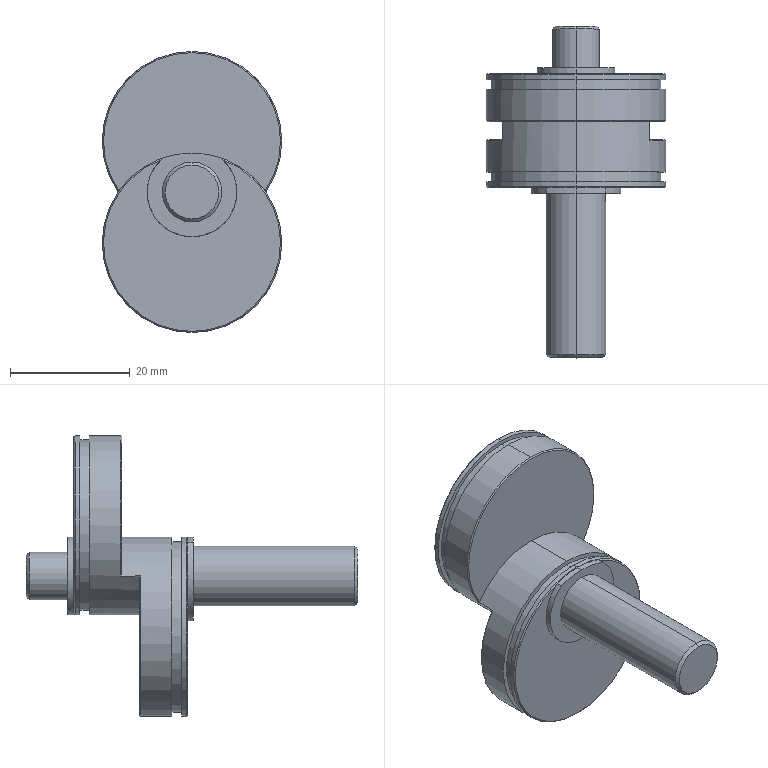Part | SolidWorks | features ICE 7, Chamfer 2, BaseBody 1 | 1 solid | 47 faces | box 30 x 55.5 x 47 mm | volume 14567 mm3 | cylinder 21 | cone 13 | plane 13 | commonest cylinder face diameters 30 x10 28.5 x4 8 x2 10 x2 13 x2 15 x1
STEP:
#1=CARTESIAN_POINT('',(0.,0.,-4.5));
#2=VERTEX_POINT('',#1);
#3=CARTESIAN_POINT('',(0.,0.,4.5));
#4=VERTEX_POINT('',#3);
#5=CARTESIAN_POINT('',(0.,0.,0.));
#6=DIRECTION('',(0.,-1.,0.));
#7=DIRECTION('',(0.,0.,-1.));
#8=AXIS2_PLACEMENT_3D('',#5,#6,#7);
#9=CIRCLE('',#8,4.5);
#10=EDGE_CURVE('',#2,#4,#9,.T.);
#11=ORIENTED_EDGE('',*,*,#10,.F.);
#12=CARTESIAN_POINT('',(0.,0.5,-5.));
#13=VERTEX_POINT('',#12);
#14=CARTESIAN_POINT('',(0.,0.,-4.5));
#15=DIRECTION('',(0.,0.7071,-0.7071));
#16=VECTOR('',#15,1000.);
#17=LINE('',#14,#16);
#18=EDGE_CURVE('',#2,#13,#17,.T.);
#19=ORIENTED_EDGE('',*,*,#18,.T.);
#20=CARTESIAN_POINT('',(0.,0.5,5.));
#21=VERTEX_POINT('',#20);
#22=CARTESIAN_POINT('',(0.,0.5,0.));
#23=DIRECTION('',(0.,1.,0.));
#24=DIRECTION('',(0.,0.,-1.));
#25=AXIS2_PLACEMENT_3D('',#22,#23,#24);
#26=CIRCLE('',#25,5.);
#27=EDGE_CURVE('',#21,#13,#26,.T.);
#28=ORIENTED_EDGE('',*,*,#27,.F.);
#29=CARTESIAN_POINT('',(0.,0.,4.5));
#30=DIRECTION('',(0.,0.7071,0.7071));
#31=VECTOR('',#30,1000.);
#32=LINE('',#29,#31);
#33=EDGE_CURVE('',#4,#21,#32,.T.);
#34=ORIENTED_EDGE('',*,*,#33,.F.);
#35=EDGE_LOOP('',(#11,#19,#28,#34));
#36=FACE_OUTER_BOUND('',#35,.T.);
#37=CARTESIAN_POINT('',(0.,0.,0.));
#38=DIRECTION('',(0.,1.,0.));
#39=DIRECTION('',(0.,0.,1.));
#40=AXIS2_PLACEMENT_3D('',#37,#38,#39);
#41=CONICAL_SURFACE('',#40,4.5,0.7854);
#42=ADVANCED_FACE('',(#36),#41,.T.);
#43=CARTESIAN_POINT('',(0.,55.5,3.5));
#44=VERTEX_POINT('',#43);
#45=CARTESIAN_POINT('',(0.,55.5,-3.5));
#46=VERTEX_POINT('',#45);
#47=CARTESIAN_POINT('',(0.,55.5,0.));
#48=DIRECTION('',(0.,1.,0.));
#49=DIRECTION('',(0.,0.,1.));
#50=AXIS2_PLACEMENT_3D('',#47,#48,#49);
#51=CIRCLE('',#50,3.5);
#52=EDGE_CURVE('',#44,#46,#51,.T.);
#53=ORIENTED_EDGE('',*,*,#52,.F.);
#54=CARTESIAN_POINT('',(0.,55.,4.));
#55=VERTEX_POINT('',#54);
#56=CARTESIAN_POINT('',(0.,55.5,3.5));
#57=DIRECTION('',(0.,-0.7071,0.7071));
#58=VECTOR('',#57,1000.);
#59=LINE('',#56,#58);
#60=EDGE_CURVE('',#44,#55,#59,.T.);
#61=ORIENTED_EDGE('',*,*,#60,.T.);
#62=CARTESIAN_POINT('',(0.,55.,-4.));
#63=VERTEX_POINT('',#62);
#64=CARTESIAN_POINT('',(0.,55.,0.));
#65=DIRECTION('',(0.,-1.,0.));
#66=DIRECTION('',(0.,0.,1.));
#67=AXIS2_PLACEMENT_3D('',#64,#65,#66);
#68=CIRCLE('',#67,4.);
#69=EDGE_CURVE('',#63,#55,#68,.T.);
#70=ORIENTED_EDGE('',*,*,#69,.F.);
#71=CARTESIAN_POINT('',(0.,55.5,-3.5));
#72=DIRECTION('',(0.,-0.7071,-0.7071));
#73=VECTOR('',#72,1000.);
#74=LINE('',#71,#73);
#75=EDGE_CURVE('',#46,#63,#74,.T.);
#76=ORIENTED_EDGE('',*,*,#75,.F.);
#77=EDGE_LOOP('',(#53,#61,#70,#76));
#78=FACE_OUTER_BOUND('',#77,.T.);
#79=CARTESIAN_POINT('',(0.,55.5,0.));
#80=DIRECTION('',(0.,-1.,0.));
#81=DIRECTION('',(0.,0.,-1.));
#82=AXIS2_PLACEMENT_3D('',#79,#80,#81);
#83=CONICAL_SURFACE('',#82,3.5,0.7854);
#84=ADVANCED_FACE('',(#78),#83,.T.);
#85=ORIENTED_EDGE('',*,*,#69,.T.);
#86=CARTESIAN_POINT('',(0.,48.5,4.));
#87=VERTEX_POINT('',#86);
#88=CARTESIAN_POINT('',(0.,55.5,4.));
#89=DIRECTION('',(0.,-1.,0.));
#90=VECTOR('',#89,1000.);
#91=LINE('',#88,#90);
#92=EDGE_CURVE('',#55,#87,#91,.T.);
#93=ORIENTED_EDGE('',*,*,#92,.T.);
#94=CARTESIAN_POINT('',(0.,48.5,-4.));
#95=VERTEX_POINT('',#94);
#96=CARTESIAN_POINT('',(0.,48.5,0.));
#97=DIRECTION('',(0.,1.,0.));
#98=DIRECTION('',(0.,0.,1.));
#99=AXIS2_PLACEMENT_3D('',#96,#97,#98);
#100=CIRCLE('',#99,4.);
#101=EDGE_CURVE('',#87,#95,#100,.T.);
#102=ORIENTED_EDGE('',*,*,#101,.T.);
#103=CARTESIAN_POINT('',(0.,55.5,-4.));
#104=DIRECTION('',(0.,-1.,0.));
#105=VECTOR('',#104,1000.);
#106=LINE('',#103,#105);
#107=EDGE_CURVE('',#63,#95,#106,.T.);
#108=ORIENTED_EDGE('',*,*,#107,.F.);
#109=EDGE_LOOP('',(#85,#93,#102,#108));
#110=FACE_OUTER_BOUND('',#109,.T.);
#111=CARTESIAN_POINT('',(0.,55.5,0.));
#112=DIRECTION('',(0.,-1.,0.));
#113=DIRECTION('',(0.,0.,-1.));
#114=AXIS2_PLACEMENT_3D('',#111,#112,#113);
#115=CYLINDRICAL_SURFACE('',#114,4.);
#116=ADVANCED_FACE('',(#110),#115,.T.);
#117=ORIENTED_EDGE('',*,*,#27,.T.);
#118=CARTESIAN_POINT('',(0.,27.5,-5.));
#119=VERTEX_POINT('',#118);
#120=CARTESIAN_POINT('',(0.,0.,-5.));
#121=DIRECTION('',(0.,1.,0.));
#122=VECTOR('',#121,1000.);
#123=LINE('',#120,#122);
#124=EDGE_CURVE('',#13,#119,#123,.T.);
#125=ORIENTED_EDGE('',*,*,#124,.T.);
#126=CARTESIAN_POINT('',(0.,27.5,5.));
#127=VERTEX_POINT('',#126);
#128=CARTESIAN_POINT('',(0.,27.5,0.));
#129=DIRECTION('',(0.,-1.,0.));
#130=DIRECTION('',(0.,0.,-1.));
#131=AXIS2_PLACEMENT_3D('',#128,#129,#130);
#132=CIRCLE('',#131,5.);
#133=EDGE_CURVE('',#119,#127,#132,.T.);
#134=ORIENTED_EDGE('',*,*,#133,.T.);
#135=CARTESIAN_POINT('',(0.,0.,5.));
#136=DIRECTION('',(0.,1.,0.));
#137=VECTOR('',#136,1000.);
#138=LINE('',#135,#137);
#139=EDGE_CURVE('',#21,#127,#138,.T.);
#140=ORIENTED_EDGE('',*,*,#139,.F.);
#141=EDGE_LOOP('',(#117,#125,#134,#140));
#142=FACE_OUTER_BOUND('',#141,.T.);
#143=CARTESIAN_POINT('',(0.,0.,0.));
#144=DIRECTION('',(0.,1.,0.));
#145=DIRECTION('',(0.,0.,1.));
#146=AXIS2_PLACEMENT_3D('',#143,#144,#145);
#147=CYLINDRICAL_SURFACE('',#146,5.);
#148=ADVANCED_FACE('',(#142),#147,.T.);
#149=CARTESIAN_POINT('',(0.,27.5,6.5));
#150=VERTEX_POINT('',#149);
#151=CARTESIAN_POINT('',(-4.902,27.5,5.676));
#152=VERTEX_POINT('',#151);
#153=CARTESIAN_POINT('',(0.,27.5,-8.5));
#154=DIRECTION('',(0.,-1.,0.));
#155=DIRECTION('',(0.,0.,1.));
#156=AXIS2_PLACEMENT_3D('',#153,#154,#155);
#157=CIRCLE('',#156,15.);
#158=EDGE_CURVE('',#150,#152,#157,.T.);
#159=ORIENTED_EDGE('',*,*,#158,.F.);
#160=CARTESIAN_POINT('',(0.,28.5,6.5));
#161=VERTEX_POINT('',#160);
#162=CARTESIAN_POINT('',(0.,27.5,6.5));
#163=DIRECTION('',(0.,1.,0.));
#164=VECTOR('',#163,1000.);
#165=LINE('',#162,#164);
#166=EDGE_CURVE('',#150,#161,#165,.T.);
#167=ORIENTED_EDGE('',*,*,#166,.T.);
#168=CARTESIAN_POINT('',(-4.902,28.5,5.676));
#169=VERTEX_POINT('',#168);
#170=CARTESIAN_POINT('',(0.,28.5,-8.5));
#171=DIRECTION('',(0.,-1.,0.));
#172=DIRECTION('',(0.,0.,1.));
#173=AXIS2_PLACEMENT_3D('',#170,#171,#172);
#174=CIRCLE('',#173,15.);
#175=EDGE_CURVE('',#161,#169,#174,.T.);
#176=ORIENTED_EDGE('',*,*,#175,.T.);
#177=CARTESIAN_POINT('',(-4.902,27.5,5.676));
#178=DIRECTION('',(0.,1.,0.));
#179=VECTOR('',#178,1000.);
#180=LINE('',#177,#179);
#181=EDGE_CURVE('',#152,#169,#180,.T.);
#182=ORIENTED_EDGE('',*,*,#181,.F.);
#183=EDGE_LOOP('',(#159,#167,#176,#182));
#184=FACE_OUTER_BOUND('',#183,.T.);
#185=CARTESIAN_POINT('',(0.,27.5,-8.5));
#186=DIRECTION('',(0.,1.,0.));
#187=DIRECTION('',(0.,0.,1.));
#188=AXIS2_PLACEMENT_3D('',#185,#186,#187);
#189=CYLINDRICAL_SURFACE('',#188,15.);
#190=ADVANCED_FACE('',(#184),#189,.T.);
#191=CARTESIAN_POINT('',(0.,28.5,-23.3));
#192=VERTEX_POINT('',#191);
#193=CARTESIAN_POINT('',(5.281,28.5,5.326));
#194=VERTEX_POINT('',#193);
#195=CARTESIAN_POINT('',(0.,28.5,-8.5));
#196=DIRECTION('',(0.,-1.,0.));
#197=DIRECTION('',(0.,0.,-1.));
#198=AXIS2_PLACEMENT_3D('',#195,#196,#197);
#199=CIRCLE('',#198,14.8);
#200=EDGE_CURVE('',#192,#194,#199,.T.);
#201=ORIENTED_EDGE('',*,*,#200,.F.);
#202=CARTESIAN_POINT('',(0.,28.7,-23.5));
#203=VERTEX_POINT('',#202);
#204=CARTESIAN_POINT('',(0.,28.7,-23.5));
#205=DIRECTION('',(0.,0.7071,-0.7071));
#206=VECTOR('',#205,1000.);
#207=LINE('',#204,#206);
#208=EDGE_CURVE('',#192,#203,#207,.T.);
#209=ORIENTED_EDGE('',*,*,#208,.T.);
#210=CARTESIAN_POINT('',(0.,28.7,6.5));
#211=VERTEX_POINT('',#210);
#212=CARTESIAN_POINT('',(0.,28.7,-8.5));
#213=DIRECTION('',(0.,1.,0.));
#214=DIRECTION('',(0.,0.,-1.));
#215=AXIS2_PLACEMENT_3D('',#212,#213,#214);
#216=CIRCLE('',#215,15.);
#217=EDGE_CURVE('',#211,#203,#216,.T.);
#218=ORIENTED_EDGE('',*,*,#217,.F.);
#219=CARTESIAN_POINT('',(0.,28.5,6.3));
#220=VERTEX_POINT('',#219);
#221=CARTESIAN_POINT('',(0.,28.7,6.5));
#222=DIRECTION('',(0.,0.7071,0.7071));
#223=VECTOR('',#222,1000.);
#224=LINE('',#221,#223);
#225=EDGE_CURVE('',#220,#211,#224,.T.);
#226=ORIENTED_EDGE('',*,*,#225,.F.);
#227=CARTESIAN_POINT('',(0.,28.5,-8.5));
#228=DIRECTION('',(0.,-1.,0.));
#229=DIRECTION('',(0.,0.,-1.));
#230=AXIS2_PLACEMENT_3D('',#227,#228,#229);
#231=CIRCLE('',#230,14.8);
#232=EDGE_CURVE('',#194,#220,#231,.T.);
#233=ORIENTED_EDGE('',*,*,#232,.F.);
#234=EDGE_LOOP('',(#201,#209,#218,#226,#233));
#235=FACE_OUTER_BOUND('',#234,.T.);
#236=CARTESIAN_POINT('',(0.,28.7,-8.5));
#237=DIRECTION('',(0.,1.,0.));
#238=DIRECTION('',(0.,0.,1.));
#239=AXIS2_PLACEMENT_3D('',#236,#237,#238);
#240=CONICAL_SURFACE('',#239,15.,0.7854);
#241=ADVANCED_FACE('',(#235),#240,.T.);
#242=ORIENTED_EDGE('',*,*,#217,.T.);
#243=CARTESIAN_POINT('',(0.,29.5,-23.5));
#244=VERTEX_POINT('',#243);
#245=CARTESIAN_POINT('',(0.,28.5,-23.5));
#246=DIRECTION('',(0.,1.,0.));
#247=VECTOR('',#246,1000.);
#248=LINE('',#245,#247);
#249=EDGE_CURVE('',#203,#244,#248,.T.);
#250=ORIENTED_EDGE('',*,*,#249,.T.);
#251=CARTESIAN_POINT('',(0.,29.5,6.5));
#252=VERTEX_POINT('',#251);
#253=CARTESIAN_POINT('',(0.,29.5,-8.5));
#254=DIRECTION('',(0.,1.,0.));
#255=DIRECTION('',(0.,0.,-1.));
#256=AXIS2_PLACEMENT_3D('',#253,#254,#255);
#257=CIRCLE('',#256,15.);
#258=EDGE_CURVE('',#252,#244,#257,.T.);
#259=ORIENTED_EDGE('',*,*,#258,.F.);
#260=CARTESIAN_POINT('',(0.,28.5,6.5));
#261=DIRECTION('',(0.,1.,0.));
#262=VECTOR('',#261,1000.);
#263=LINE('',#260,#262);
#264=EDGE_CURVE('',#211,#252,#263,.T.);
#265=ORIENTED_EDGE('',*,*,#264,.F.);
#266=EDGE_LOOP('',(#242,#250,#259,#265));
#267=FACE_OUTER_BOUND('',#266,.T.);
#268=CARTESIAN_POINT('',(0.,28.5,-8.5));
#269=DIRECTION('',(0.,1.,0.));
#270=DIRECTION('',(0.,0.,1.));
#271=AXIS2_PLACEMENT_3D('',#268,#269,#270);
#272=CYLINDRICAL_SURFACE('',#271,15.);
#273=ADVANCED_FACE('',(#267),#272,.T.);
#274=CARTESIAN_POINT('',(0.,29.5,-22.75));
#275=VERTEX_POINT('',#274);
#276=CARTESIAN_POINT('',(0.,29.5,5.75));
#277=VERTEX_POINT('',#276);
#278=CARTESIAN_POINT('',(0.,29.5,-8.5));
#279=DIRECTION('',(0.,-1.,0.));
#280=DIRECTION('',(0.,0.,-1.));
#281=AXIS2_PLACEMENT_3D('',#278,#279,#280);
#282=CIRCLE('',#281,14.25);
#283=EDGE_CURVE('',#275,#277,#282,.T.);
#284=ORIENTED_EDGE('',*,*,#283,.F.);
#285=CARTESIAN_POINT('',(0.,31.1,-22.75));
#286=VERTEX_POINT('',#285);
#287=CARTESIAN_POINT('',(0.,29.5,-22.75));
#288=DIRECTION('',(0.,1.,0.));
#289=VECTOR('',#288,1000.);
#290=LINE('',#287,#289);
#291=EDGE_CURVE('',#275,#286,#290,.T.);
#292=ORIENTED_EDGE('',*,*,#291,.T.);
#293=CARTESIAN_POINT('',(0.,31.1,5.75));
#294=VERTEX_POINT('',#293);
#295=CARTESIAN_POINT('',(0.,31.1,-8.5));
#296=DIRECTION('',(0.,-1.,0.));
#297=DIRECTION('',(0.,0.,-1.));
#298=AXIS2_PLACEMENT_3D('',#295,#296,#297);
#299=CIRCLE('',#298,14.25);
#300=EDGE_CURVE('',#286,#294,#299,.T.);
#301=ORIENTED_EDGE('',*,*,#300,.T.);
#302=CARTESIAN_POINT('',(0.,29.5,5.75));
#303=DIRECTION('',(0.,1.,0.));
#304=VECTOR('',#303,1000.);
#305=LINE('',#302,#304);
#306=EDGE_CURVE('',#277,#294,#305,.T.);
#307=ORIENTED_EDGE('',*,*,#306,.F.);
#308=EDGE_LOOP('',(#284,#292,#301,#307));
#309=FACE_OUTER_BOUND('',#308,.T.);
#310=CARTESIAN_POINT('',(0.,29.5,-8.5));
#311=DIRECTION('',(0.,1.,0.));
#312=DIRECTION('',(0.,0.,1.));
#313=AXIS2_PLACEMENT_3D('',#310,#311,#312);
#314=CYLINDRICAL_SURFACE('',#313,14.25);
#315=ADVANCED_FACE('',(#309),#314,.T.);
#316=CARTESIAN_POINT('',(14.8,47.5,8.5));
#317=VERTEX_POINT('',#316);
#318=CARTESIAN_POINT('',(-14.8,47.5,8.5));
#319=VERTEX_POINT('',#318);
#320=CARTESIAN_POINT('',(0.,47.5,8.5));
#321=DIRECTION('',(0.,-1.,0.));
#322=DIRECTION('',(1.,0.,0.));
#323=AXIS2_PLACEMENT_3D('',#320,#321,#322);
#324=CIRCLE('',#323,14.8);
#325=EDGE_CURVE('',#317,#319,#324,.T.);
#326=ORIENTED_EDGE('',*,*,#325,.T.);
#327=CARTESIAN_POINT('',(-15.,47.3,8.5));
#328=VERTEX_POINT('',#327);
#329=CARTESIAN_POINT('',(-15.,47.3,8.5));
#330=DIRECTION('',(-0.7071,-0.7071,0.));
#331=VECTOR('',#330,1000.);
#332=LINE('',#329,#331);
#333=EDGE_CURVE('',#319,#328,#332,.T.);
#334=ORIENTED_EDGE('',*,*,#333,.T.);
#335=CARTESIAN_POINT('',(0.,47.3,23.5));
#336=VERTEX_POINT('',#335);
#337=CARTESIAN_POINT('',(0.,47.3,8.5));
#338=DIRECTION('',(0.,1.,0.));
#339=DIRECTION('',(0.,0.,-1.));
#340=AXIS2_PLACEMENT_3D('',#337,#338,#339);
#341=CIRCLE('',#340,15.);
#342=EDGE_CURVE('',#328,#336,#341,.T.);
#343=ORIENTED_EDGE('',*,*,#342,.T.);
#344=CARTESIAN_POINT('',(15.,47.3,8.5));
#345=VERTEX_POINT('',#344);
#346=CARTESIAN_POINT('',(0.,47.3,8.5));
#347=DIRECTION('',(0.,1.,0.));
#348=DIRECTION('',(0.,0.,-1.));
#349=AXIS2_PLACEMENT_3D('',#346,#347,#348);
#350=CIRCLE('',#349,15.);
#351=EDGE_CURVE('',#336,#345,#350,.T.);
#352=ORIENTED_EDGE('',*,*,#351,.T.);
#353=CARTESIAN_POINT('',(15.,47.3,8.5));
#354=DIRECTION('',(0.7071,-0.7071,0.));
#355=VECTOR('',#354,1000.);
#356=LINE('',#353,#355);
#357=EDGE_CURVE('',#317,#345,#356,.T.);
#358=ORIENTED_EDGE('',*,*,#357,.F.);
#359=EDGE_LOOP('',(#326,#334,#343,#352,#358));
#360=FACE_OUTER_BOUND('',#359,.T.);
#361=CARTESIAN_POINT('',(0.,47.3,8.5));
#362=DIRECTION('',(0.,-1.,0.));
#363=DIRECTION('',(1.,0.,0.));
#364=AXIS2_PLACEMENT_3D('',#361,#362,#363);
#365=CONICAL_SURFACE('',#364,15.,0.7854);
#366=ADVANCED_FACE('',(#360),#365,.T.);
#367=CARTESIAN_POINT('',(2.106,47.5,-6.149));
#368=VERTEX_POINT('',#367);
#369=CARTESIAN_POINT('',(0.,47.5,8.5));
#370=DIRECTION('',(0.,-1.,0.));
#371=DIRECTION('',(1.,0.,0.));
#372=AXIS2_PLACEMENT_3D('',#369,#370,#371);
#373=CIRCLE('',#372,14.8);
#374=EDGE_CURVE('',#368,#317,#373,.T.);
#375=ORIENTED_EDGE('',*,*,#374,.T.);
#376=ORIENTED_EDGE('',*,*,#357,.T.);
#377=CARTESIAN_POINT('',(0.0001635,47.3,-6.5));
#378=VERTEX_POINT('',#377);
#379=CARTESIAN_POINT('',(0.,47.3,8.5));
#380=DIRECTION('',(0.,1.,0.));
#381=DIRECTION('',(0.,0.,-1.));
#382=AXIS2_PLACEMENT_3D('',#379,#380,#381);
#383=CIRCLE('',#382,15.);
#384=EDGE_CURVE('',#345,#378,#383,.T.);
#385=ORIENTED_EDGE('',*,*,#384,.T.);
#386=CARTESIAN_POINT('',(0.0001635,47.3,-6.5));
#387=CARTESIAN_POINT('',(0.7279,47.3,-6.5));
#388=CARTESIAN_POINT('',(1.429,47.367,-6.381));
#389=CARTESIAN_POINT('',(2.106,47.5,-6.149));
#390=B_SPLINE_CURVE_WITH_KNOTS('',3,(#386,#387,#388,#389),.UNSPECIFIED.,.F.,.F.,(4,4),(0.,0.002144),.UNSPECIFIED.);
#391=EDGE_CURVE('',#378,#368,#390,.T.);
#392=ORIENTED_EDGE('',*,*,#391,.T.);
#393=EDGE_LOOP('',(#375,#376,#385,#392));
#394=FACE_OUTER_BOUND('',#393,.T.);
#395=CARTESIAN_POINT('',(0.,47.3,8.5));
#396=DIRECTION('',(0.,-1.,0.));
#397=DIRECTION('',(1.,0.,0.));
#398=AXIS2_PLACEMENT_3D('',#395,#396,#397);
#399=CONICAL_SURFACE('',#398,15.,0.7854);
#400=ADVANCED_FACE('',(#394),#399,.T.);
#401=ORIENTED_EDGE('',*,*,#351,.F.);
#402=CARTESIAN_POINT('',(0.,46.5,23.5));
#403=VERTEX_POINT('',#402);
#404=CARTESIAN_POINT('',(0.,47.5,23.5));
#405=DIRECTION('',(0.,-1.,0.));
#406=VECTOR('',#405,1000.);
#407=LINE('',#404,#406);
#408=EDGE_CURVE('',#336,#403,#407,.T.);
#409=ORIENTED_EDGE('',*,*,#408,.T.);
#410=CARTESIAN_POINT('',(0.,46.5,-6.5));
#411=VERTEX_POINT('',#410);
#412=CARTESIAN_POINT('',(0.,46.5,8.5));
#413=DIRECTION('',(0.,1.,0.));
#414=DIRECTION('',(0.,0.,-1.));
#415=AXIS2_PLACEMENT_3D('',#412,#413,#414);
#416=CIRCLE('',#415,15.);
#417=EDGE_CURVE('',#403,#411,#416,.T.);
#418=ORIENTED_EDGE('',*,*,#417,.T.);
#419=CARTESIAN_POINT('',(0.,47.3,-6.5));
#420=VERTEX_POINT('',#419);
#421=CARTESIAN_POINT('',(0.,47.5,-6.5));
#422=DIRECTION('',(0.,-1.,0.));
#423=VECTOR('',#422,1000.);
#424=LINE('',#421,#423);
#425=EDGE_CURVE('',#420,#411,#424,.T.);
#426=ORIENTED_EDGE('',*,*,#425,.F.);
#427=CARTESIAN_POINT('',(0.,47.3,8.5));
#428=DIRECTION('',(0.,1.,0.));
#429=DIRECTION('',(-0.000000001,0.,-1.));
#430=AXIS2_PLACEMENT_3D('',#427,#428,#429);
#431=CIRCLE('',#430,15.);
#432=EDGE_CURVE('',#378,#420,#431,.T.);
#433=ORIENTED_EDGE('',*,*,#432,.F.);
#434=ORIENTED_EDGE('',*,*,#384,.F.);
#435=EDGE_LOOP('',(#401,#409,#418,#426,#433,#434));
#436=FACE_OUTER_BOUND('',#435,.T.);
#437=CARTESIAN_POINT('',(0.,47.5,8.5));
#438=DIRECTION('',(0.,-1.,0.));
#439=DIRECTION('',(0.,0.,-1.));
#440=AXIS2_PLACEMENT_3D('',#437,#438,#439);
#441=CYLINDRICAL_SURFACE('',#440,15.);
#442=ADVANCED_FACE('',(#436),#441,.T.);
#443=CARTESIAN_POINT('',(0.,44.9,22.75));
#444=VERTEX_POINT('',#443);
#445=CARTESIAN_POINT('',(0.,44.9,-5.75));
#446=VERTEX_POINT('',#445);
#447=CARTESIAN_POINT('',(0.,44.9,8.5));
#448=DIRECTION('',(0.,1.,0.));
#449=DIRECTION('',(0.,0.,1.));
#450=AXIS2_PLACEMENT_3D('',#447,#448,#449);
#451=CIRCLE('',#450,14.25);
#452=EDGE_CURVE('',#444,#446,#451,.T.);
#453=ORIENTED_EDGE('',*,*,#452,.T.);
#454=CARTESIAN_POINT('',(0.,46.5,-5.75));
#455=VERTEX_POINT('',#454);
#456=CARTESIAN_POINT('',(0.,46.5,-5.75));
#457=DIRECTION('',(0.,1.,0.));
#458=VECTOR('',#457,1000.);
#459=LINE('',#456,#458);
#460=EDGE_CURVE('',#446,#455,#459,.T.);
#461=ORIENTED_EDGE('',*,*,#460,.T.);
#462=CARTESIAN_POINT('',(0.,46.5,22.75));
#463=VERTEX_POINT('',#462);
#464=CARTESIAN_POINT('',(0.,46.5,8.5));
#465=DIRECTION('',(0.,-1.,0.));
#466=DIRECTION('',(0.,0.,1.));
#467=AXIS2_PLACEMENT_3D('',#464,#465,#466);
#468=CIRCLE('',#467,14.25);
#469=EDGE_CURVE('',#455,#463,#468,.T.);
#470=ORIENTED_EDGE('',*,*,#469,.T.);
#471=CARTESIAN_POINT('',(0.,46.5,22.75));
#472=DIRECTION('',(0.,1.,0.));
#473=VECTOR('',#472,1000.);
#474=LINE('',#471,#473);
#475=EDGE_CURVE('',#444,#463,#474,.T.);
#476=ORIENTED_EDGE('',*,*,#475,.F.);
#477=EDGE_LOOP('',(#453,#461,#470,#476));
#478=FACE_OUTER_BOUND('',#477,.T.);
#479=CARTESIAN_POINT('',(0.,46.5,8.5));
#480=DIRECTION('',(0.,1.,0.));
#481=DIRECTION('',(0.,0.,1.));
#482=AXIS2_PLACEMENT_3D('',#479,#480,#481);
#483=CYLINDRICAL_SURFACE('',#482,14.25);
#484=ADVANCED_FACE('',(#478),#483,.T.);
#485=CARTESIAN_POINT('',(0.,44.9,23.5));
#486=VERTEX_POINT('',#485);
#487=CARTESIAN_POINT('',(0.,44.9,-6.5));
#488=VERTEX_POINT('',#487);
#489=CARTESIAN_POINT('',(0.,44.9,8.5));
#490=DIRECTION('',(0.,1.,0.));
#491=DIRECTION('',(0.,0.,-1.));
#492=AXIS2_PLACEMENT_3D('',#489,#490,#491);
#493=CIRCLE('',#492,15.);
#494=EDGE_CURVE('',#486,#488,#493,.T.);
#495=ORIENTED_EDGE('',*,*,#494,.F.);
#496=CARTESIAN_POINT('',(0.,39.7,23.5));
#497=VERTEX_POINT('',#496);
#498=CARTESIAN_POINT('',(0.,47.5,23.5));
#499=DIRECTION('',(0.,-1.,0.));
#500=VECTOR('',#499,1000.);
#501=LINE('',#498,#500);
#502=EDGE_CURVE('',#486,#497,#501,.T.);
#503=ORIENTED_EDGE('',*,*,#502,.T.);
#504=CARTESIAN_POINT('',(12.359,39.7,0.));
#505=VERTEX_POINT('',#504);
#506=CARTESIAN_POINT('',(0.,39.7,8.5));
#507=DIRECTION('',(0.,1.,0.));
#508=DIRECTION('',(0.,0.,-1.));
#509=AXIS2_PLACEMENT_3D('',#506,#507,#508);
#510=CIRCLE('',#509,15.);
#511=EDGE_CURVE('',#497,#505,#510,.T.);
#512=ORIENTED_EDGE('',*,*,#511,.T.);
#513=CARTESIAN_POINT('',(12.359,36.3,0.));
#514=VERTEX_POINT('',#513);
#515=CARTESIAN_POINT('',(12.359,47.5,0.));
#516=DIRECTION('',(0.,-1.,0.));
#517=VECTOR('',#516,1000.);
#518=LINE('',#515,#517);
#519=EDGE_CURVE('',#505,#514,#518,.T.);
#520=ORIENTED_EDGE('',*,*,#519,.T.);
#521=CARTESIAN_POINT('',(12.237,36.5,-0.1753));
#522=VERTEX_POINT('',#521);
#523=CARTESIAN_POINT('',(12.237,36.5,-0.1753));
#524=CARTESIAN_POINT('',(12.278,36.433,-0.1172));
#525=CARTESIAN_POINT('',(12.319,36.367,-0.05877));
#526=CARTESIAN_POINT('',(12.359,36.3,0.));
#527=B_SPLINE_CURVE_WITH_KNOTS('',3,(#523,#524,#525,#526),.UNSPECIFIED.,.F.,.F.,(4,4),(0.,0.0002928),.UNSPECIFIED.);
#528=EDGE_CURVE('',#522,#514,#527,.T.);
#529=ORIENTED_EDGE('',*,*,#528,.F.);
#530=CARTESIAN_POINT('',(0.,36.5,-6.5));
#531=VERTEX_POINT('',#530);
#532=CARTESIAN_POINT('',(0.,36.5,8.5));
#533=DIRECTION('',(0.,1.,0.));
#534=DIRECTION('',(0.,0.,-1.));
#535=AXIS2_PLACEMENT_3D('',#532,#533,#534);
#536=CIRCLE('',#535,15.);
#537=EDGE_CURVE('',#522,#531,#536,.T.);
#538=ORIENTED_EDGE('',*,*,#537,.T.);
#539=CARTESIAN_POINT('',(0.,47.5,-6.5));
#540=DIRECTION('',(0.,-1.,0.));
#541=VECTOR('',#540,1000.);
#542=LINE('',#539,#541);
#543=EDGE_CURVE('',#488,#531,#542,.T.);
#544=ORIENTED_EDGE('',*,*,#543,.F.);
#545=EDGE_LOOP('',(#495,#503,#512,#520,#529,#538,#544));
#546=FACE_OUTER_BOUND('',#545,.T.);
#547=CARTESIAN_POINT('',(0.,47.5,8.5));
#548=DIRECTION('',(0.,-1.,0.));
#549=DIRECTION('',(0.,0.,-1.));
#550=AXIS2_PLACEMENT_3D('',#547,#548,#549);
#551=CYLINDRICAL_SURFACE('',#550,15.);
#552=ADVANCED_FACE('',(#546),#551,.T.);
#553=CARTESIAN_POINT('',(-12.237,39.5,0.1753));
#554=VERTEX_POINT('',#553);
#555=CARTESIAN_POINT('',(0.,39.5,23.3));
#556=VERTEX_POINT('',#555);
#557=CARTESIAN_POINT('',(0.,39.5,8.5));
#558=DIRECTION('',(0.,1.,0.));
#559=DIRECTION('',(0.,0.,1.));
#560=AXIS2_PLACEMENT_3D('',#557,#558,#559);
#561=CIRCLE('',#560,14.8);
#562=EDGE_CURVE('',#554,#556,#561,.T.);
#563=ORIENTED_EDGE('',*,*,#562,.T.);
#564=CARTESIAN_POINT('',(0.,39.7,23.5));
#565=DIRECTION('',(0.,0.7071,0.7071));
#566=VECTOR('',#565,1000.);
#567=LINE('',#564,#566);
#568=EDGE_CURVE('',#556,#497,#567,.T.);
#569=ORIENTED_EDGE('',*,*,#568,.T.);
#570=CARTESIAN_POINT('',(-12.359,39.7,0.));
#571=VERTEX_POINT('',#570);
#572=CARTESIAN_POINT('',(0.,39.7,8.5));
#573=DIRECTION('',(0.,1.,0.));
#574=DIRECTION('',(0.,0.,-1.));
#575=AXIS2_PLACEMENT_3D('',#572,#573,#574);
#576=CIRCLE('',#575,15.);
#577=EDGE_CURVE('',#571,#497,#576,.T.);
#578=ORIENTED_EDGE('',*,*,#577,.F.);
#579=CARTESIAN_POINT('',(-12.359,39.7,0.));
#580=CARTESIAN_POINT('',(-12.319,39.633,0.05877));
#581=CARTESIAN_POINT('',(-12.278,39.567,0.1172));
#582=CARTESIAN_POINT('',(-12.237,39.5,0.1753));
#583=B_SPLINE_CURVE_WITH_KNOTS('',3,(#579,#580,#581,#582),.UNSPECIFIED.,.F.,.F.,(4,4),(0.,0.0002928),.UNSPECIFIED.);
#584=EDGE_CURVE('',#571,#554,#583,.T.);
#585=ORIENTED_EDGE('',*,*,#584,.T.);
#586=EDGE_LOOP('',(#563,#569,#578,#585));
#587=FACE_OUTER_BOUND('',#586,.T.);
#588=CARTESIAN_POINT('',(0.,39.7,8.5));
#589=DIRECTION('',(0.,1.,0.));
#590=DIRECTION('',(0.,0.,1.));
#591=AXIS2_PLACEMENT_3D('',#588,#589,#590);
#592=CONICAL_SURFACE('',#591,15.,0.7854);
#593=ADVANCED_FACE('',(#587),#592,.T.);
#594=CARTESIAN_POINT('',(-12.237,36.5,-0.1753));
#595=VERTEX_POINT('',#594);
#596=CARTESIAN_POINT('',(0.,36.5,-23.3));
#597=VERTEX_POINT('',#596);
#598=CARTESIAN_POINT('',(0.,36.5,-8.5));
#599=DIRECTION('',(0.,-1.,0.));
#600=DIRECTION('',(0.,0.,-1.));
#601=AXIS2_PLACEMENT_3D('',#598,#599,#600);
#602=CIRCLE('',#601,14.8);
#603=EDGE_CURVE('',#595,#597,#602,.T.);
#604=ORIENTED_EDGE('',*,*,#603,.T.);
#605=CARTESIAN_POINT('',(0.,36.3,-23.5));
#606=VERTEX_POINT('',#605);
#607=CARTESIAN_POINT('',(0.,36.3,-23.5));
#608=DIRECTION('',(0.,-0.7071,-0.7071));
#609=VECTOR('',#608,1000.);
#610=LINE('',#607,#609);
#611=EDGE_CURVE('',#597,#606,#610,.T.);
#612=ORIENTED_EDGE('',*,*,#611,.T.);
#613=CARTESIAN_POINT('',(-12.359,36.3,0.));
#614=VERTEX_POINT('',#613);
#615=CARTESIAN_POINT('',(0.,36.3,-8.5));
#616=DIRECTION('',(0.,1.,0.));
#617=DIRECTION('',(0.,0.,-1.));
#618=AXIS2_PLACEMENT_3D('',#615,#616,#617);
#619=CIRCLE('',#618,15.);
#620=EDGE_CURVE('',#606,#614,#619,.T.);
#621=ORIENTED_EDGE('',*,*,#620,.T.);
#622=CARTESIAN_POINT('',(-12.237,36.5,-0.1753));
#623=CARTESIAN_POINT('',(-12.278,36.433,-0.1172));
#624=CARTESIAN_POINT('',(-12.319,36.367,-0.05877));
#625=CARTESIAN_POINT('',(-12.359,36.3,0.));
#626=B_SPLINE_CURVE_WITH_KNOTS('',3,(#622,#623,#624,#625),.UNSPECIFIED.,.F.,.F.,(4,4),(0.,0.0002928),.UNSPECIFIED.);
#627=EDGE_CURVE('',#595,#614,#626,.T.);
#628=ORIENTED_EDGE('',*,*,#627,.F.);
#629=EDGE_LOOP('',(#604,#612,#621,#628));
#630=FACE_OUTER_BOUND('',#629,.T.);
#631=CARTESIAN_POINT('',(0.,36.3,-8.5));
#632=DIRECTION('',(0.,-1.,0.));
#633=DIRECTION('',(0.,0.,-1.));
#634=AXIS2_PLACEMENT_3D('',#631,#632,#633);
#635=CONICAL_SURFACE('',#634,15.,0.7854);
#636=ADVANCED_FACE('',(#630),#635,.T.);
#637=CARTESIAN_POINT('',(0.,47.3,-6.5));
#638=VERTEX_POINT('',#637);
#639=CARTESIAN_POINT('',(0.0001635,47.3,-6.5));
#640=CARTESIAN_POINT('',(0.000109,47.3,-6.5));
#641=CARTESIAN_POINT('',(0.0000545,47.3,-6.5));
#642=CARTESIAN_POINT('',(0.,47.3,-6.5));
#643=B_SPLINE_CURVE_WITH_KNOTS('',3,(#639,#640,#641,#642),.UNSPECIFIED.,.F.,.F.,(4,4),(0.,0.000000161),.UNSPECIFIED.);
#644=EDGE_CURVE('',#378,#638,#643,.T.);
#645=ORIENTED_EDGE('',*,*,#644,.T.);
#646=CARTESIAN_POINT('',(0.,48.5,-6.5));
#647=VERTEX_POINT('',#646);
#648=CARTESIAN_POINT('',(0.,48.5,-6.5));
#649=DIRECTION('',(0.,1.,0.));
#650=VECTOR('',#649,1000.);
#651=LINE('',#648,#650);
#652=EDGE_CURVE('',#638,#647,#651,.T.);
#653=ORIENTED_EDGE('',*,*,#652,.T.);
#654=CARTESIAN_POINT('',(0.,48.5,6.5));
#655=VERTEX_POINT('',#654);
#656=CARTESIAN_POINT('',(0.,48.5,0.));
#657=DIRECTION('',(0.,1.,0.));
#658=DIRECTION('',(0.,0.,1.));
#659=AXIS2_PLACEMENT_3D('',#656,#657,#658);
#660=CIRCLE('',#659,6.5);
#661=EDGE_CURVE('',#655,#647,#660,.T.);
#662=ORIENTED_EDGE('',*,*,#661,.F.);
#663=CARTESIAN_POINT('',(0.,47.5,6.5));
#664=VERTEX_POINT('',#663);
#665=CARTESIAN_POINT('',(0.,48.5,6.5));
#666=DIRECTION('',(0.,1.,0.));
#667=VECTOR('',#666,1000.);
#668=LINE('',#665,#667);
#669=EDGE_CURVE('',#664,#655,#668,.T.);
#670=ORIENTED_EDGE('',*,*,#669,.F.);
#671=CARTESIAN_POINT('',(0.,47.5,0.));
#672=DIRECTION('',(0.,1.,0.));
#673=DIRECTION('',(0.,0.,-1.));
#674=AXIS2_PLACEMENT_3D('',#671,#672,#673);
#675=CIRCLE('',#674,6.5);
#676=EDGE_CURVE('',#664,#368,#675,.T.);
#677=ORIENTED_EDGE('',*,*,#676,.T.);
#678=ORIENTED_EDGE('',*,*,#391,.F.);
#679=EDGE_LOOP('',(#645,#653,#662,#670,#677,#678));
#680=FACE_OUTER_BOUND('',#679,.T.);
#681=CARTESIAN_POINT('',(0.,48.5,0.));
#682=DIRECTION('',(0.,1.,0.));
#683=DIRECTION('',(0.,0.,1.));
#684=AXIS2_PLACEMENT_3D('',#681,#682,#683);
#685=CYLINDRICAL_SURFACE('',#684,6.5);
#686=ADVANCED_FACE('',(#680),#685,.T.);
#687=CARTESIAN_POINT('',(12.237,39.5,0.1753));
#688=VERTEX_POINT('',#687);
#689=CARTESIAN_POINT('',(0.,39.5,6.5));
#690=VERTEX_POINT('',#689);
#691=CARTESIAN_POINT('',(0.,39.5,-8.5));
#692=DIRECTION('',(0.,-1.,0.));
#693=DIRECTION('',(0.,0.,-1.));
#694=AXIS2_PLACEMENT_3D('',#691,#692,#693);
#695=CIRCLE('',#694,15.);
#696=EDGE_CURVE('',#688,#690,#695,.T.);
#697=ORIENTED_EDGE('',*,*,#696,.T.);
#698=CARTESIAN_POINT('',(0.,31.1,6.5));
#699=VERTEX_POINT('',#698);
#700=CARTESIAN_POINT('',(0.,39.5,6.5));
#701=DIRECTION('',(0.,-1.,0.));
#702=VECTOR('',#701,1000.);
#703=LINE('',#700,#702);
#704=EDGE_CURVE('',#690,#699,#703,.T.);
#705=ORIENTED_EDGE('',*,*,#704,.T.);
#706=CARTESIAN_POINT('',(0.,31.1,-23.5));
#707=VERTEX_POINT('',#706);
#708=CARTESIAN_POINT('',(0.,31.1,-8.5));
#709=DIRECTION('',(0.,-1.,0.));
#710=DIRECTION('',(0.,0.,-1.));
#711=AXIS2_PLACEMENT_3D('',#708,#709,#710);
#712=CIRCLE('',#711,15.);
#713=EDGE_CURVE('',#707,#699,#712,.T.);
#714=ORIENTED_EDGE('',*,*,#713,.F.);
#715=CARTESIAN_POINT('',(0.,39.5,-23.5));
#716=DIRECTION('',(0.,-1.,0.));
#717=VECTOR('',#716,1000.);
#718=LINE('',#715,#717);
#719=EDGE_CURVE('',#606,#707,#718,.T.);
#720=ORIENTED_EDGE('',*,*,#719,.F.);
#721=CARTESIAN_POINT('',(0.,36.3,-8.5));
#722=DIRECTION('',(0.,1.,0.));
#723=DIRECTION('',(0.,0.,-1.));
#724=AXIS2_PLACEMENT_3D('',#721,#722,#723);
#725=CIRCLE('',#724,15.);
#726=EDGE_CURVE('',#514,#606,#725,.T.);
#727=ORIENTED_EDGE('',*,*,#726,.F.);
#728=ORIENTED_EDGE('',*,*,#519,.F.);
#729=CARTESIAN_POINT('',(12.359,39.7,0.));
#730=CARTESIAN_POINT('',(12.319,39.633,0.05877));
#731=CARTESIAN_POINT('',(12.278,39.567,0.1172));
#732=CARTESIAN_POINT('',(12.237,39.5,0.1753));
#733=B_SPLINE_CURVE_WITH_KNOTS('',3,(#729,#730,#731,#732),.UNSPECIFIED.,.F.,.F.,(4,4),(0.,0.0002928),.UNSPECIFIED.);
#734=EDGE_CURVE('',#505,#688,#733,.T.);
#735=ORIENTED_EDGE('',*,*,#734,.T.);
#736=EDGE_LOOP('',(#697,#705,#714,#720,#727,#728,#735));
#737=FACE_OUTER_BOUND('',#736,.T.);
#738=CARTESIAN_POINT('',(0.,39.5,-8.5));
#739=DIRECTION('',(0.,-1.,0.));
#740=DIRECTION('',(0.,0.,-1.));
#741=AXIS2_PLACEMENT_3D('',#738,#739,#740);
#742=CYLINDRICAL_SURFACE('',#741,15.);
#743=ADVANCED_FACE('',(#737),#742,.T.);
#744=CARTESIAN_POINT('',(-2.106,47.5,-6.149));
#745=VERTEX_POINT('',#744);
#746=CARTESIAN_POINT('',(0.,47.5,0.));
#747=DIRECTION('',(0.,1.,0.));
#748=DIRECTION('',(0.,0.,-1.));
#749=AXIS2_PLACEMENT_3D('',#746,#747,#748);
#750=CIRCLE('',#749,6.5);
#751=EDGE_CURVE('',#745,#664,#750,.T.);
#752=ORIENTED_EDGE('',*,*,#751,.F.);
#753=CARTESIAN_POINT('',(0.,47.5,8.5));
#754=DIRECTION('',(0.,-1.,0.));
#755=DIRECTION('',(1.,0.,0.));
#756=AXIS2_PLACEMENT_3D('',#753,#754,#755);
#757=CIRCLE('',#756,14.8);
#758=EDGE_CURVE('',#319,#745,#757,.T.);
#759=ORIENTED_EDGE('',*,*,#758,.F.);
#760=ORIENTED_EDGE('',*,*,#325,.F.);
#761=ORIENTED_EDGE('',*,*,#374,.F.);
#762=ORIENTED_EDGE('',*,*,#676,.F.);
#763=EDGE_LOOP('',(#752,#759,#760,#761,#762));
#764=FACE_OUTER_BOUND('',#763,.T.);
#765=CARTESIAN_POINT('',(0.,47.5,0.));
#766=DIRECTION('',(0.,-1.,0.));
#767=DIRECTION('',(0.,0.,-1.));
#768=AXIS2_PLACEMENT_3D('',#765,#766,#767);
#769=PLANE('',#768);
#770=ADVANCED_FACE('',(#764),#769,.F.);
#771=ORIENTED_EDGE('',*,*,#704,.F.);
#772=CARTESIAN_POINT('',(0.,39.5,-8.5));
#773=DIRECTION('',(0.,-1.,0.));
#774=DIRECTION('',(0.,0.,-1.));
#775=AXIS2_PLACEMENT_3D('',#772,#773,#774);
#776=CIRCLE('',#775,15.);
#777=EDGE_CURVE('',#690,#554,#776,.T.);
#778=ORIENTED_EDGE('',*,*,#777,.T.);
#779=ORIENTED_EDGE('',*,*,#584,.F.);
#780=CARTESIAN_POINT('',(-12.359,47.5,0.));
#781=DIRECTION('',(0.,1.,0.));
#782=VECTOR('',#781,1000.);
#783=LINE('',#780,#782);
#784=EDGE_CURVE('',#614,#571,#783,.T.);
#785=ORIENTED_EDGE('',*,*,#784,.F.);
#786=ORIENTED_EDGE('',*,*,#620,.F.);
#787=ORIENTED_EDGE('',*,*,#719,.T.);
#788=CARTESIAN_POINT('',(0.,31.1,-8.5));
#789=DIRECTION('',(0.,-1.,0.));
#790=DIRECTION('',(0.,0.,-1.));
#791=AXIS2_PLACEMENT_3D('',#788,#789,#790);
#792=CIRCLE('',#791,15.);
#793=EDGE_CURVE('',#699,#707,#792,.T.);
#794=ORIENTED_EDGE('',*,*,#793,.F.);
#795=EDGE_LOOP('',(#771,#778,#779,#785,#786,#787,#794));
#796=FACE_OUTER_BOUND('',#795,.T.);
#797=CARTESIAN_POINT('',(0.,39.5,-8.5));
#798=DIRECTION('',(0.,-1.,0.));
#799=DIRECTION('',(0.,0.,-1.));
#800=AXIS2_PLACEMENT_3D('',#797,#798,#799);
#801=CYLINDRICAL_SURFACE('',#800,15.);
#802=ADVANCED_FACE('',(#796),#801,.T.);
#803=ORIENTED_EDGE('',*,*,#652,.F.);
#804=CARTESIAN_POINT('',(0.,47.3,-6.5));
#805=CARTESIAN_POINT('',(-0.7277,47.3,-6.5));
#806=CARTESIAN_POINT('',(-1.429,47.367,-6.381));
#807=CARTESIAN_POINT('',(-2.106,47.5,-6.149));
#808=B_SPLINE_CURVE_WITH_KNOTS('',3,(#804,#805,#806,#807),.UNSPECIFIED.,.F.,.F.,(4,4),(0.000000161,0.002144),.UNSPECIFIED.);
#809=EDGE_CURVE('',#638,#745,#808,.T.);
#810=ORIENTED_EDGE('',*,*,#809,.T.);
#811=ORIENTED_EDGE('',*,*,#751,.T.);
#812=ORIENTED_EDGE('',*,*,#669,.T.);
#813=CARTESIAN_POINT('',(0.,48.5,0.));
#814=DIRECTION('',(0.,1.,0.));
#815=DIRECTION('',(0.,0.,1.));
#816=AXIS2_PLACEMENT_3D('',#813,#814,#815);
#817=CIRCLE('',#816,6.5);
#818=EDGE_CURVE('',#647,#655,#817,.T.);
#819=ORIENTED_EDGE('',*,*,#818,.F.);
#820=EDGE_LOOP('',(#803,#810,#811,#812,#819));
#821=FACE_OUTER_BOUND('',#820,.T.);
#822=CARTESIAN_POINT('',(0.,48.5,0.));
#823=DIRECTION('',(0.,1.,0.));
#824=DIRECTION('',(0.,0.,1.));
#825=AXIS2_PLACEMENT_3D('',#822,#823,#824);
#826=CYLINDRICAL_SURFACE('',#825,6.5);
#827=ADVANCED_FACE('',(#821),#826,.T.);
#828=ORIENTED_EDGE('',*,*,#333,.F.);
#829=ORIENTED_EDGE('',*,*,#758,.T.);
#830=ORIENTED_EDGE('',*,*,#809,.F.);
#831=ORIENTED_EDGE('',*,*,#644,.F.);
#832=ORIENTED_EDGE('',*,*,#432,.T.);
#833=CARTESIAN_POINT('',(0.,47.3,8.5));
#834=DIRECTION('',(0.,1.,0.));
#835=DIRECTION('',(0.,0.,-1.));
#836=AXIS2_PLACEMENT_3D('',#833,#834,#835);
#837=CIRCLE('',#836,15.);
#838=EDGE_CURVE('',#420,#328,#837,.T.);
#839=ORIENTED_EDGE('',*,*,#838,.T.);
#840=EDGE_LOOP('',(#828,#829,#830,#831,#832,#839));
#841=FACE_OUTER_BOUND('',#840,.T.);
#842=CARTESIAN_POINT('',(0.,47.3,8.5));
#843=DIRECTION('',(0.,-1.,0.));
#844=DIRECTION('',(1.,0.,0.));
#845=AXIS2_PLACEMENT_3D('',#842,#843,#844);
#846=CONICAL_SURFACE('',#845,15.,0.7854);
#847=ADVANCED_FACE('',(#841),#846,.T.);
#848=ORIENTED_EDGE('',*,*,#408,.F.);
#849=ORIENTED_EDGE('',*,*,#342,.F.);
#850=ORIENTED_EDGE('',*,*,#838,.F.);
#851=ORIENTED_EDGE('',*,*,#425,.T.);
#852=CARTESIAN_POINT('',(0.,46.5,8.5));
#853=DIRECTION('',(0.,1.,0.));
#854=DIRECTION('',(0.,0.,-1.));
#855=AXIS2_PLACEMENT_3D('',#852,#853,#854);
#856=CIRCLE('',#855,15.);
#857=EDGE_CURVE('',#411,#403,#856,.T.);
#858=ORIENTED_EDGE('',*,*,#857,.T.);
#859=EDGE_LOOP('',(#848,#849,#850,#851,#858));
#860=FACE_OUTER_BOUND('',#859,.T.);
#861=CARTESIAN_POINT('',(0.,47.5,8.5));
#862=DIRECTION('',(0.,-1.,0.));
#863=DIRECTION('',(0.,0.,-1.));
#864=AXIS2_PLACEMENT_3D('',#861,#862,#863);
#865=CYLINDRICAL_SURFACE('',#864,15.);
#866=ADVANCED_FACE('',(#860),#865,.T.);
#867=ORIENTED_EDGE('',*,*,#857,.F.);
#868=ORIENTED_EDGE('',*,*,#417,.F.);
#869=EDGE_LOOP('',(#867,#868));
#870=FACE_OUTER_BOUND('',#869,.T.);
#871=CARTESIAN_POINT('',(0.,46.5,8.5));
#872=DIRECTION('',(0.,-1.,0.));
#873=DIRECTION('',(0.,0.,1.));
#874=AXIS2_PLACEMENT_3D('',#871,#872,#873);
#875=CIRCLE('',#874,14.25);
#876=EDGE_CURVE('',#463,#455,#875,.T.);
#877=ORIENTED_EDGE('',*,*,#876,.F.);
#878=ORIENTED_EDGE('',*,*,#469,.F.);
#879=EDGE_LOOP('',(#877,#878));
#880=FACE_BOUND('',#879,.T.);
#881=CARTESIAN_POINT('',(0.,46.5,0.));
#882=DIRECTION('',(0.,1.,0.));
#883=DIRECTION('',(0.,0.,1.));
#884=AXIS2_PLACEMENT_3D('',#881,#882,#883);
#885=PLANE('',#884);
#886=ADVANCED_FACE('',(#870,#880),#885,.F.);
#887=ORIENTED_EDGE('',*,*,#460,.F.);
#888=CARTESIAN_POINT('',(0.,44.9,8.5));
#889=DIRECTION('',(0.,1.,0.));
#890=DIRECTION('',(0.,0.,1.));
#891=AXIS2_PLACEMENT_3D('',#888,#889,#890);
#892=CIRCLE('',#891,14.25);
#893=EDGE_CURVE('',#446,#444,#892,.T.);
#894=ORIENTED_EDGE('',*,*,#893,.T.);
#895=ORIENTED_EDGE('',*,*,#475,.T.);
#896=ORIENTED_EDGE('',*,*,#876,.T.);
#897=EDGE_LOOP('',(#887,#894,#895,#896));
#898=FACE_OUTER_BOUND('',#897,.T.);
#899=CARTESIAN_POINT('',(0.,46.5,8.5));
#900=DIRECTION('',(0.,1.,0.));
#901=DIRECTION('',(0.,0.,1.));
#902=AXIS2_PLACEMENT_3D('',#899,#900,#901);
#903=CYLINDRICAL_SURFACE('',#902,14.25);
#904=ADVANCED_FACE('',(#898),#903,.T.);
#905=CARTESIAN_POINT('',(0.,44.9,8.5));
#906=DIRECTION('',(0.,1.,0.));
#907=DIRECTION('',(0.,0.,-1.));
#908=AXIS2_PLACEMENT_3D('',#905,#906,#907);
#909=CIRCLE('',#908,15.);
#910=EDGE_CURVE('',#488,#486,#909,.T.);
#911=ORIENTED_EDGE('',*,*,#910,.T.);
#912=ORIENTED_EDGE('',*,*,#494,.T.);
#913=EDGE_LOOP('',(#911,#912));
#914=FACE_OUTER_BOUND('',#913,.T.);
#915=ORIENTED_EDGE('',*,*,#452,.F.);
#916=ORIENTED_EDGE('',*,*,#893,.F.);
#917=EDGE_LOOP('',(#915,#916));
#918=FACE_BOUND('',#917,.T.);
#919=CARTESIAN_POINT('',(0.,44.9,0.));
#920=DIRECTION('',(0.,1.,0.));
#921=DIRECTION('',(0.,0.,1.));
#922=AXIS2_PLACEMENT_3D('',#919,#920,#921);
#923=PLANE('',#922);
#924=ADVANCED_FACE('',(#914,#918),#923,.T.);
#925=ORIENTED_EDGE('',*,*,#502,.F.);
#926=ORIENTED_EDGE('',*,*,#910,.F.);
#927=ORIENTED_EDGE('',*,*,#543,.T.);
#928=CARTESIAN_POINT('',(0.,36.5,8.5));
#929=DIRECTION('',(0.,1.,0.));
#930=DIRECTION('',(0.,0.,-1.));
#931=AXIS2_PLACEMENT_3D('',#928,#929,#930);
#932=CIRCLE('',#931,15.);
#933=EDGE_CURVE('',#531,#595,#932,.T.);
#934=ORIENTED_EDGE('',*,*,#933,.T.);
#935=ORIENTED_EDGE('',*,*,#627,.T.);
#936=ORIENTED_EDGE('',*,*,#784,.T.);
#937=ORIENTED_EDGE('',*,*,#577,.T.);
#938=EDGE_LOOP('',(#925,#926,#927,#934,#935,#936,#937));
#939=FACE_OUTER_BOUND('',#938,.T.);
#940=CARTESIAN_POINT('',(0.,47.5,8.5));
#941=DIRECTION('',(0.,-1.,0.));
#942=DIRECTION('',(0.,0.,-1.));
#943=AXIS2_PLACEMENT_3D('',#940,#941,#942);
#944=CYLINDRICAL_SURFACE('',#943,15.);
#945=ADVANCED_FACE('',(#939),#944,.T.);
#946=ORIENTED_EDGE('',*,*,#603,.F.);
#947=ORIENTED_EDGE('',*,*,#933,.F.);
#948=ORIENTED_EDGE('',*,*,#537,.F.);
#949=CARTESIAN_POINT('',(0.,36.5,-8.5));
#950=DIRECTION('',(0.,-1.,0.));
#951=DIRECTION('',(0.,0.,-1.));
#952=AXIS2_PLACEMENT_3D('',#949,#950,#951);
#953=CIRCLE('',#952,14.8);
#954=EDGE_CURVE('',#597,#522,#953,.T.);
#955=ORIENTED_EDGE('',*,*,#954,.F.);
#956=EDGE_LOOP('',(#946,#947,#948,#955));
#957=FACE_OUTER_BOUND('',#956,.T.);
#958=CARTESIAN_POINT('',(0.,36.5,0.));
#959=DIRECTION('',(0.,-1.,0.));
#960=DIRECTION('',(0.,0.,-1.));
#961=AXIS2_PLACEMENT_3D('',#958,#959,#960);
#962=PLANE('',#961);
#963=ADVANCED_FACE('',(#957),#962,.F.);
#964=ORIENTED_EDGE('',*,*,#568,.F.);
#965=CARTESIAN_POINT('',(0.,39.5,8.5));
#966=DIRECTION('',(0.,1.,0.));
#967=DIRECTION('',(0.,0.,1.));
#968=AXIS2_PLACEMENT_3D('',#965,#966,#967);
#969=CIRCLE('',#968,14.8);
#970=EDGE_CURVE('',#556,#688,#969,.T.);
#971=ORIENTED_EDGE('',*,*,#970,.T.);
#972=ORIENTED_EDGE('',*,*,#734,.F.);
#973=ORIENTED_EDGE('',*,*,#511,.F.);
#974=EDGE_LOOP('',(#964,#971,#972,#973));
#975=FACE_OUTER_BOUND('',#974,.T.);
#976=CARTESIAN_POINT('',(0.,39.7,8.5));
#977=DIRECTION('',(0.,1.,0.));
#978=DIRECTION('',(0.,0.,1.));
#979=AXIS2_PLACEMENT_3D('',#976,#977,#978);
#980=CONICAL_SURFACE('',#979,15.,0.7854);
#981=ADVANCED_FACE('',(#975),#980,.T.);
#982=ORIENTED_EDGE('',*,*,#611,.F.);
#983=ORIENTED_EDGE('',*,*,#954,.T.);
#984=ORIENTED_EDGE('',*,*,#528,.T.);
#985=ORIENTED_EDGE('',*,*,#726,.T.);
#986=EDGE_LOOP('',(#982,#983,#984,#985));
#987=FACE_OUTER_BOUND('',#986,.T.);
#988=CARTESIAN_POINT('',(0.,36.3,-8.5));
#989=DIRECTION('',(0.,-1.,0.));
#990=DIRECTION('',(0.,0.,-1.));
#991=AXIS2_PLACEMENT_3D('',#988,#989,#990);
#992=CONICAL_SURFACE('',#991,15.,0.7854);
#993=ADVANCED_FACE('',(#987),#992,.T.);
#994=ORIENTED_EDGE('',*,*,#562,.F.);
#995=ORIENTED_EDGE('',*,*,#777,.F.);
#996=ORIENTED_EDGE('',*,*,#696,.F.);
#997=ORIENTED_EDGE('',*,*,#970,.F.);
#998=EDGE_LOOP('',(#994,#995,#996,#997));
#999=FACE_OUTER_BOUND('',#998,.T.);
#1000=CARTESIAN_POINT('',(0.,39.5,0.));
#1001=DIRECTION('',(0.,-1.,0.));
#1002=DIRECTION('',(0.,0.,-1.));
#1003=AXIS2_PLACEMENT_3D('',#1000,#1001,#1002);
#1004=PLANE('',#1003);
#1005=ADVANCED_FACE('',(#999),#1004,.T.);
#1006=CARTESIAN_POINT('',(0.,31.1,-8.5));
#1007=DIRECTION('',(0.,-1.,0.));
#1008=DIRECTION('',(0.,0.,-1.));
#1009=AXIS2_PLACEMENT_3D('',#1006,#1007,#1008);
#1010=CIRCLE('',#1009,14.25);
#1011=EDGE_CURVE('',#294,#286,#1010,.T.);
#1012=ORIENTED_EDGE('',*,*,#1011,.F.);
#1013=ORIENTED_EDGE('',*,*,#300,.F.);
#1014=EDGE_LOOP('',(#1012,#1013));
#1015=FACE_BOUND('',#1014,.T.);
#1016=ORIENTED_EDGE('',*,*,#713,.T.);
#1017=ORIENTED_EDGE('',*,*,#793,.T.);
#1018=EDGE_LOOP('',(#1016,#1017));
#1019=FACE_OUTER_BOUND('',#1018,.T.);
#1020=CARTESIAN_POINT('',(0.,31.1,-8.5));
#1021=DIRECTION('',(0.,-1.,0.));
#1022=DIRECTION('',(0.,0.,-1.));
#1023=AXIS2_PLACEMENT_3D('',#1020,#1021,#1022);
#1024=PLANE('',#1023);
#1025=ADVANCED_FACE('',(#1015,#1019),#1024,.T.);
#1026=ORIENTED_EDGE('',*,*,#291,.F.);
#1027=CARTESIAN_POINT('',(0.,29.5,-8.5));
#1028=DIRECTION('',(0.,-1.,0.));
#1029=DIRECTION('',(0.,0.,-1.));
#1030=AXIS2_PLACEMENT_3D('',#1027,#1028,#1029);
#1031=CIRCLE('',#1030,14.25);
#1032=EDGE_CURVE('',#277,#275,#1031,.T.);
#1033=ORIENTED_EDGE('',*,*,#1032,.F.);
#1034=ORIENTED_EDGE('',*,*,#306,.T.);
#1035=ORIENTED_EDGE('',*,*,#1011,.T.);
#1036=EDGE_LOOP('',(#1026,#1033,#1034,#1035));
#1037=FACE_OUTER_BOUND('',#1036,.T.);
#1038=CARTESIAN_POINT('',(0.,29.5,-8.5));
#1039=DIRECTION('',(0.,1.,0.));
#1040=DIRECTION('',(0.,0.,1.));
#1041=AXIS2_PLACEMENT_3D('',#1038,#1039,#1040);
#1042=CYLINDRICAL_SURFACE('',#1041,14.25);
#1043=ADVANCED_FACE('',(#1037),#1042,.T.);
#1044=ORIENTED_EDGE('',*,*,#249,.F.);
#1045=CARTESIAN_POINT('',(0.,28.7,-8.5));
#1046=DIRECTION('',(0.,1.,0.));
#1047=DIRECTION('',(0.,0.,-1.));
#1048=AXIS2_PLACEMENT_3D('',#1045,#1046,#1047);
#1049=CIRCLE('',#1048,15.);
#1050=EDGE_CURVE('',#203,#211,#1049,.T.);
#1051=ORIENTED_EDGE('',*,*,#1050,.T.);
#1052=ORIENTED_EDGE('',*,*,#264,.T.);
#1053=CARTESIAN_POINT('',(0.,29.5,-8.5));
#1054=DIRECTION('',(0.,1.,0.));
#1055=DIRECTION('',(0.,0.,-1.));
#1056=AXIS2_PLACEMENT_3D('',#1053,#1054,#1055);
#1057=CIRCLE('',#1056,15.);
#1058=EDGE_CURVE('',#244,#252,#1057,.T.);
#1059=ORIENTED_EDGE('',*,*,#1058,.F.);
#1060=EDGE_LOOP('',(#1044,#1051,#1052,#1059));
#1061=FACE_OUTER_BOUND('',#1060,.T.);
#1062=CARTESIAN_POINT('',(0.,28.5,-8.5));
#1063=DIRECTION('',(0.,1.,0.));
#1064=DIRECTION('',(0.,0.,1.));
#1065=AXIS2_PLACEMENT_3D('',#1062,#1063,#1064);
#1066=CYLINDRICAL_SURFACE('',#1065,15.);
#1067=ADVANCED_FACE('',(#1061),#1066,.T.);
#1068=CARTESIAN_POINT('',(-5.281,28.5,5.326));
#1069=VERTEX_POINT('',#1068);
#1070=CARTESIAN_POINT('',(0.,28.5,0.));
#1071=DIRECTION('',(0.,-1.,0.));
#1072=DIRECTION('',(0.,0.,1.));
#1073=AXIS2_PLACEMENT_3D('',#1070,#1071,#1072);
#1074=CIRCLE('',#1073,7.5);
#1075=EDGE_CURVE('',#1069,#194,#1074,.T.);
#1076=ORIENTED_EDGE('',*,*,#1075,.F.);
#1077=CARTESIAN_POINT('',(0.,28.5,-8.5));
#1078=DIRECTION('',(0.,-1.,0.));
#1079=DIRECTION('',(0.,0.,-1.));
#1080=AXIS2_PLACEMENT_3D('',#1077,#1078,#1079);
#1081=CIRCLE('',#1080,14.8);
#1082=EDGE_CURVE('',#1069,#192,#1081,.T.);
#1083=ORIENTED_EDGE('',*,*,#1082,.T.);
#1084=ORIENTED_EDGE('',*,*,#200,.T.);
#1085=EDGE_LOOP('',(#1076,#1083,#1084));
#1086=FACE_OUTER_BOUND('',#1085,.T.);
#1087=CARTESIAN_POINT('',(0.,28.5,-8.5));
#1088=DIRECTION('',(0.,-1.,0.));
#1089=DIRECTION('',(0.,0.,-1.));
#1090=AXIS2_PLACEMENT_3D('',#1087,#1088,#1089);
#1091=PLANE('',#1090);
#1092=ADVANCED_FACE('',(#1086),#1091,.T.);
#1093=ORIENTED_EDGE('',*,*,#1032,.T.);
#1094=ORIENTED_EDGE('',*,*,#283,.T.);
#1095=EDGE_LOOP('',(#1093,#1094));
#1096=FACE_BOUND('',#1095,.T.);
#1097=ORIENTED_EDGE('',*,*,#258,.T.);
#1098=ORIENTED_EDGE('',*,*,#1058,.T.);
#1099=EDGE_LOOP('',(#1097,#1098));
#1100=FACE_OUTER_BOUND('',#1099,.T.);
#1101=CARTESIAN_POINT('',(0.,29.5,-8.5));
#1102=DIRECTION('',(0.,-1.,0.));
#1103=DIRECTION('',(0.,0.,-1.));
#1104=AXIS2_PLACEMENT_3D('',#1101,#1102,#1103);
#1105=PLANE('',#1104);
#1106=ADVANCED_FACE('',(#1096,#1100),#1105,.F.);
#1107=ORIENTED_EDGE('',*,*,#208,.F.);
#1108=ORIENTED_EDGE('',*,*,#1082,.F.);
#1109=CARTESIAN_POINT('',(0.,28.5,-8.5));
#1110=DIRECTION('',(0.,-1.,0.));
#1111=DIRECTION('',(0.,0.,-1.));
#1112=AXIS2_PLACEMENT_3D('',#1109,#1110,#1111);
#1113=CIRCLE('',#1112,14.8);
#1114=EDGE_CURVE('',#220,#1069,#1113,.T.);
#1115=ORIENTED_EDGE('',*,*,#1114,.F.);
#1116=ORIENTED_EDGE('',*,*,#225,.T.);
#1117=ORIENTED_EDGE('',*,*,#1050,.F.);
#1118=EDGE_LOOP('',(#1107,#1108,#1115,#1116,#1117));
#1119=FACE_OUTER_BOUND('',#1118,.T.);
#1120=CARTESIAN_POINT('',(0.,28.7,-8.5));
#1121=DIRECTION('',(0.,1.,0.));
#1122=DIRECTION('',(0.,0.,1.));
#1123=AXIS2_PLACEMENT_3D('',#1120,#1121,#1122);
#1124=CONICAL_SURFACE('',#1123,15.,0.7854);
#1125=ADVANCED_FACE('',(#1119),#1124,.T.);
#1126=ORIENTED_EDGE('',*,*,#166,.F.);
#1127=CARTESIAN_POINT('',(4.902,27.5,5.676));
#1128=VERTEX_POINT('',#1127);
#1129=CARTESIAN_POINT('',(0.,27.5,-8.5));
#1130=DIRECTION('',(0.,-1.,0.));
#1131=DIRECTION('',(0.,0.,1.));
#1132=AXIS2_PLACEMENT_3D('',#1129,#1130,#1131);
#1133=CIRCLE('',#1132,15.);
#1134=EDGE_CURVE('',#1128,#150,#1133,.T.);
#1135=ORIENTED_EDGE('',*,*,#1134,.F.);
#1136=CARTESIAN_POINT('',(4.902,28.5,5.676));
#1137=VERTEX_POINT('',#1136);
#1138=CARTESIAN_POINT('',(4.902,27.5,5.676));
#1139=DIRECTION('',(0.,1.,0.));
#1140=VECTOR('',#1139,1000.);
#1141=LINE('',#1138,#1140);
#1142=EDGE_CURVE('',#1128,#1137,#1141,.T.);
#1143=ORIENTED_EDGE('',*,*,#1142,.T.);
#1144=CARTESIAN_POINT('',(0.,28.5,-8.5));
#1145=DIRECTION('',(0.,-1.,0.));
#1146=DIRECTION('',(0.,0.,1.));
#1147=AXIS2_PLACEMENT_3D('',#1144,#1145,#1146);
#1148=CIRCLE('',#1147,15.);
#1149=EDGE_CURVE('',#1137,#161,#1148,.T.);
#1150=ORIENTED_EDGE('',*,*,#1149,.T.);
#1151=EDGE_LOOP('',(#1126,#1135,#1143,#1150));
#1152=FACE_OUTER_BOUND('',#1151,.T.);
#1153=CARTESIAN_POINT('',(0.,27.5,-8.5));
#1154=DIRECTION('',(0.,1.,0.));
#1155=DIRECTION('',(0.,0.,1.));
#1156=AXIS2_PLACEMENT_3D('',#1153,#1154,#1155);
#1157=CYLINDRICAL_SURFACE('',#1156,15.);
#1158=ADVANCED_FACE('',(#1152),#1157,.T.);
#1159=CARTESIAN_POINT('',(0.,28.5,0.));
#1160=DIRECTION('',(0.,-1.,0.));
#1161=DIRECTION('',(0.,0.,1.));
#1162=AXIS2_PLACEMENT_3D('',#1159,#1160,#1161);
#1163=CIRCLE('',#1162,7.5);
#1164=EDGE_CURVE('',#169,#1069,#1163,.T.);
#1165=ORIENTED_EDGE('',*,*,#1164,.T.);
#1166=ORIENTED_EDGE('',*,*,#1075,.T.);
#1167=CARTESIAN_POINT('',(0.,28.5,0.));
#1168=DIRECTION('',(0.,-1.,0.));
#1169=DIRECTION('',(0.,0.,1.));
#1170=AXIS2_PLACEMENT_3D('',#1167,#1168,#1169);
#1171=CIRCLE('',#1170,7.5);
#1172=EDGE_CURVE('',#194,#1137,#1171,.T.);
#1173=ORIENTED_EDGE('',*,*,#1172,.T.);
#1174=ORIENTED_EDGE('',*,*,#1142,.F.);
#1175=CARTESIAN_POINT('',(0.,27.5,0.));
#1176=DIRECTION('',(0.,-1.,0.));
#1177=DIRECTION('',(0.,0.,1.));
#1178=AXIS2_PLACEMENT_3D('',#1175,#1176,#1177);
#1179=CIRCLE('',#1178,7.5);
#1180=EDGE_CURVE('',#152,#1128,#1179,.T.);
#1181=ORIENTED_EDGE('',*,*,#1180,.F.);
#1182=ORIENTED_EDGE('',*,*,#181,.T.);
#1183=EDGE_LOOP('',(#1165,#1166,#1173,#1174,#1181,#1182));
#1184=FACE_OUTER_BOUND('',#1183,.T.);
#1185=CARTESIAN_POINT('',(0.,27.5,0.));
#1186=DIRECTION('',(0.,1.,0.));
#1187=DIRECTION('',(0.,0.,1.));
#1188=AXIS2_PLACEMENT_3D('',#1185,#1186,#1187);
#1189=CYLINDRICAL_SURFACE('',#1188,7.5);
#1190=ADVANCED_FACE('',(#1184),#1189,.T.);
#1191=CARTESIAN_POINT('',(0.,27.5,0.));
#1192=DIRECTION('',(0.,-1.,0.));
#1193=DIRECTION('',(0.,0.,-1.));
#1194=AXIS2_PLACEMENT_3D('',#1191,#1192,#1193);
#1195=CIRCLE('',#1194,5.);
#1196=EDGE_CURVE('',#127,#119,#1195,.T.);
#1197=ORIENTED_EDGE('',*,*,#1196,.F.);
#1198=ORIENTED_EDGE('',*,*,#133,.F.);
#1199=EDGE_LOOP('',(#1197,#1198));
#1200=FACE_BOUND('',#1199,.T.);
#1201=ORIENTED_EDGE('',*,*,#1134,.T.);
#1202=ORIENTED_EDGE('',*,*,#158,.T.);
#1203=ORIENTED_EDGE('',*,*,#1180,.T.);
#1204=EDGE_LOOP('',(#1201,#1202,#1203));
#1205=FACE_OUTER_BOUND('',#1204,.T.);
#1206=CARTESIAN_POINT('',(0.,27.5,-4.25));
#1207=DIRECTION('',(0.,1.,0.));
#1208=DIRECTION('',(0.,0.,1.));
#1209=AXIS2_PLACEMENT_3D('',#1206,#1207,#1208);
#1210=PLANE('',#1209);
#1211=ADVANCED_FACE('',(#1200,#1205),#1210,.F.);
#1212=ORIENTED_EDGE('',*,*,#1172,.F.);
#1213=ORIENTED_EDGE('',*,*,#232,.T.);
#1214=ORIENTED_EDGE('',*,*,#1114,.T.);
#1215=ORIENTED_EDGE('',*,*,#1164,.F.);
#1216=ORIENTED_EDGE('',*,*,#175,.F.);
#1217=ORIENTED_EDGE('',*,*,#1149,.F.);
#1218=EDGE_LOOP('',(#1212,#1213,#1214,#1215,#1216,#1217));
#1219=FACE_OUTER_BOUND('',#1218,.T.);
#1220=CARTESIAN_POINT('',(0.,28.5,-4.25));
#1221=DIRECTION('',(0.,1.,0.));
#1222=DIRECTION('',(0.,0.,1.));
#1223=AXIS2_PLACEMENT_3D('',#1220,#1221,#1222);
#1224=PLANE('',#1223);
#1225=ADVANCED_FACE('',(#1219),#1224,.T.);
#1226=CARTESIAN_POINT('',(0.,48.5,0.));
#1227=DIRECTION('',(0.,1.,0.));
#1228=DIRECTION('',(0.,0.,1.));
#1229=AXIS2_PLACEMENT_3D('',#1226,#1227,#1228);
#1230=CIRCLE('',#1229,4.);
#1231=EDGE_CURVE('',#95,#87,#1230,.T.);
#1232=ORIENTED_EDGE('',*,*,#1231,.F.);
#1233=ORIENTED_EDGE('',*,*,#101,.F.);
#1234=EDGE_LOOP('',(#1232,#1233));
#1235=FACE_BOUND('',#1234,.T.);
#1236=ORIENTED_EDGE('',*,*,#661,.T.);
#1237=ORIENTED_EDGE('',*,*,#818,.T.);
#1238=EDGE_LOOP('',(#1236,#1237));
#1239=FACE_OUTER_BOUND('',#1238,.T.);
#1240=CARTESIAN_POINT('',(0.,48.5,0.));
#1241=DIRECTION('',(0.,1.,0.));
#1242=DIRECTION('',(0.,0.,1.));
#1243=AXIS2_PLACEMENT_3D('',#1240,#1241,#1242);
#1244=PLANE('',#1243);
#1245=ADVANCED_FACE('',(#1235,#1239),#1244,.T.);
#1246=ORIENTED_EDGE('',*,*,#124,.F.);
#1247=CARTESIAN_POINT('',(0.,0.5,0.));
#1248=DIRECTION('',(0.,1.,0.));
#1249=DIRECTION('',(0.,0.,-1.));
#1250=AXIS2_PLACEMENT_3D('',#1247,#1248,#1249);
#1251=CIRCLE('',#1250,5.);
#1252=EDGE_CURVE('',#13,#21,#1251,.T.);
#1253=ORIENTED_EDGE('',*,*,#1252,.T.);
#1254=ORIENTED_EDGE('',*,*,#139,.T.);
#1255=ORIENTED_EDGE('',*,*,#1196,.T.);
#1256=EDGE_LOOP('',(#1246,#1253,#1254,#1255));
#1257=FACE_OUTER_BOUND('',#1256,.T.);
#1258=CARTESIAN_POINT('',(0.,0.,0.));
#1259=DIRECTION('',(0.,1.,0.));
#1260=DIRECTION('',(0.,0.,1.));
#1261=AXIS2_PLACEMENT_3D('',#1258,#1259,#1260);
#1262=CYLINDRICAL_SURFACE('',#1261,5.);
#1263=ADVANCED_FACE('',(#1257),#1262,.T.);
#1264=CARTESIAN_POINT('',(0.,0.,0.));
#1265=DIRECTION('',(0.,-1.,0.));
#1266=DIRECTION('',(0.,0.,-1.));
#1267=AXIS2_PLACEMENT_3D('',#1264,#1265,#1266);
#1268=CIRCLE('',#1267,4.5);
#1269=EDGE_CURVE('',#4,#2,#1268,.T.);
#1270=ORIENTED_EDGE('',*,*,#1269,.T.);
#1271=ORIENTED_EDGE('',*,*,#10,.T.);
#1272=EDGE_LOOP('',(#1270,#1271));
#1273=FACE_OUTER_BOUND('',#1272,.T.);
#1274=CARTESIAN_POINT('',(0.,0.,0.));
#1275=DIRECTION('',(0.,-1.,0.));
#1276=DIRECTION('',(0.,0.,-1.));
#1277=AXIS2_PLACEMENT_3D('',#1274,#1275,#1276);
#1278=PLANE('',#1277);
#1279=ADVANCED_FACE('',(#1273),#1278,.T.);
#1280=ORIENTED_EDGE('',*,*,#92,.F.);
#1281=CARTESIAN_POINT('',(0.,55.,0.));
#1282=DIRECTION('',(0.,-1.,0.));
#1283=DIRECTION('',(0.,0.,1.));
#1284=AXIS2_PLACEMENT_3D('',#1281,#1282,#1283);
#1285=CIRCLE('',#1284,4.);
#1286=EDGE_CURVE('',#55,#63,#1285,.T.);
#1287=ORIENTED_EDGE('',*,*,#1286,.T.);
#1288=ORIENTED_EDGE('',*,*,#107,.T.);
#1289=ORIENTED_EDGE('',*,*,#1231,.T.);
#1290=EDGE_LOOP('',(#1280,#1287,#1288,#1289));
#1291=FACE_OUTER_BOUND('',#1290,.T.);
#1292=CARTESIAN_POINT('',(0.,55.5,0.));
#1293=DIRECTION('',(0.,-1.,0.));
#1294=DIRECTION('',(0.,0.,-1.));
#1295=AXIS2_PLACEMENT_3D('',#1292,#1293,#1294);
#1296=CYLINDRICAL_SURFACE('',#1295,4.);
#1297=ADVANCED_FACE('',(#1291),#1296,.T.);
#1298=CARTESIAN_POINT('',(0.,55.5,0.));
#1299=DIRECTION('',(0.,1.,0.));
#1300=DIRECTION('',(0.,0.,1.));
#1301=AXIS2_PLACEMENT_3D('',#1298,#1299,#1300);
#1302=CIRCLE('',#1301,3.5);
#1303=EDGE_CURVE('',#46,#44,#1302,.T.);
#1304=ORIENTED_EDGE('',*,*,#1303,.T.);
#1305=ORIENTED_EDGE('',*,*,#52,.T.);
#1306=EDGE_LOOP('',(#1304,#1305));
#1307=FACE_OUTER_BOUND('',#1306,.T.);
#1308=CARTESIAN_POINT('',(0.,55.5,0.));
#1309=DIRECTION('',(0.,1.,0.));
#1310=DIRECTION('',(0.,0.,1.));
#1311=AXIS2_PLACEMENT_3D('',#1308,#1309,#1310);
#1312=PLANE('',#1311);
#1313=ADVANCED_FACE('',(#1307),#1312,.T.);
#1314=ORIENTED_EDGE('',*,*,#60,.F.);
#1315=ORIENTED_EDGE('',*,*,#1303,.F.);
#1316=ORIENTED_EDGE('',*,*,#75,.T.);
#1317=ORIENTED_EDGE('',*,*,#1286,.F.);
#1318=EDGE_LOOP('',(#1314,#1315,#1316,#1317));
#1319=FACE_OUTER_BOUND('',#1318,.T.);
#1320=CARTESIAN_POINT('',(0.,55.5,0.));
#1321=DIRECTION('',(0.,-1.,0.));
#1322=DIRECTION('',(0.,0.,-1.));
#1323=AXIS2_PLACEMENT_3D('',#1320,#1321,#1322);
#1324=CONICAL_SURFACE('',#1323,3.5,0.7854);
#1325=ADVANCED_FACE('',(#1319),#1324,.T.);
#1326=ORIENTED_EDGE('',*,*,#18,.F.);
#1327=ORIENTED_EDGE('',*,*,#1269,.F.);
#1328=ORIENTED_EDGE('',*,*,#33,.T.);
#1329=ORIENTED_EDGE('',*,*,#1252,.F.);
#1330=EDGE_LOOP('',(#1326,#1327,#1328,#1329));
#1331=FACE_OUTER_BOUND('',#1330,.T.);
#1332=CARTESIAN_POINT('',(0.,0.,0.));
#1333=DIRECTION('',(0.,1.,0.));
#1334=DIRECTION('',(0.,0.,1.));
#1335=AXIS2_PLACEMENT_3D('',#1332,#1333,#1334);
#1336=CONICAL_SURFACE('',#1335,4.5,0.7854);
#1337=ADVANCED_FACE('',(#1331),#1336,.T.);
#1338=CLOSED_SHELL('',(#42,#84,#116,#148,#190,#241,#273,#315,#366,#400,#442,#484,#552,#593,#636,#686,#743,#770,#802,#827,#847,#866,#886,#904,#924,#945,#963,#981,#993,#1005,#1025,#1043,#1067,#1092,#1106,#1125,#1158,#1190,#1211,#1225,#1245,#1263,#1279,#1297,#1313,#1325,#1337));
#1339=MANIFOLD_SOLID_BREP('',#1338);
#1340=CARTESIAN_POINT('',(0.,0.,0.));
#1341=DIRECTION('',(0.,0.,1.));
#1342=DIRECTION('',(1.,0.,0.));
#1343=AXIS2_PLACEMENT_3D('',#1340,#1341,#1342);
#1344=(LENGTH_UNIT()NAMED_UNIT(*)SI_UNIT(.MILLI.,.METRE.));
#1345=UNCERTAINTY_MEASURE_WITH_UNIT(LENGTH_MEASURE(0.00001),#1344,'','');
#1346=(NAMED_UNIT(*)PLANE_ANGLE_UNIT()SI_UNIT($,.RADIAN.));
#1347=(NAMED_UNIT(*)SI_UNIT($,.STERADIAN.)SOLID_ANGLE_UNIT());
#1348=(GEOMETRIC_REPRESENTATION_CONTEXT(3)GLOBAL_UNCERTAINTY_ASSIGNED_CONTEXT((#1345))GLOBAL_UNIT_ASSIGNED_CONTEXT((#1344,#1346,#1347))REPRESENTATION_CONTEXT('',''));
#1349=ADVANCED_BREP_SHAPE_REPRESENTATION('',(#1339,#1343),#1348);